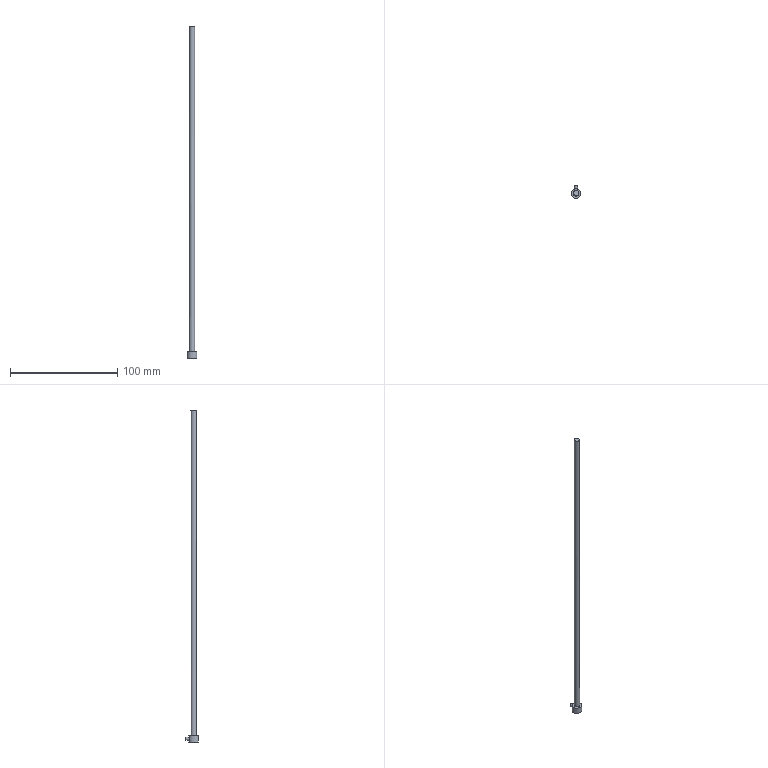Part | STEP file | E105-28-315 | 1 solid | 8 faces | box 9 x 12 x 309.813 mm | volume 6362 mm3 | cylinder 3 | plane 3 | spline 1 | cone 1 | commonest cylinder face diameters 3 x1 5 x1 9 x1
STEP:
#1=CARTESIAN_POINT('',(0.,0.,0.));
#2=DIRECTION('',(0.,0.,1.));
#3=DIRECTION('',(1.,0.,0.));
#4=AXIS2_PLACEMENT_3D('',#1,#2,#3);
#5=CARTESIAN_POINT('',(2.481,-0.3051,309.227));
#6=VERTEX_POINT('',#5);
#7=CARTESIAN_POINT('',(-2.5,0.,309.797));
#8=VERTEX_POINT('',#7);
#9=CARTESIAN_POINT('',(2.481,-0.3051,309.227));
#10=CARTESIAN_POINT('',(2.447,-0.5829,309.241));
#11=CARTESIAN_POINT('',(2.365,-0.8583,309.262));
#12=CARTESIAN_POINT('',(2.241,-1.109,309.287));
#13=CARTESIAN_POINT('',(2.117,-1.359,309.312));
#14=CARTESIAN_POINT('',(1.949,-1.591,309.342));
#15=CARTESIAN_POINT('',(1.75,-1.785,309.374));
#16=CARTESIAN_POINT('',(1.55,-1.982,309.406));
#17=CARTESIAN_POINT('',(1.313,-2.145,309.441));
#18=CARTESIAN_POINT('',(1.06,-2.264,309.476));
#19=CARTESIAN_POINT('',(0.8051,-2.383,309.511));
#20=CARTESIAN_POINT('',(0.526,-2.46,309.547));
#21=CARTESIAN_POINT('',(0.2457,-2.488,309.581));
#22=CARTESIAN_POINT('',(-0.03504,-2.516,309.615));
#23=CARTESIAN_POINT('',(-0.3247,-2.495,309.648));
#24=CARTESIAN_POINT('',(-0.5991,-2.427,309.677));
#25=CARTESIAN_POINT('',(-0.8724,-2.36,309.706));
#26=CARTESIAN_POINT('',(-1.138,-2.244,309.732));
#27=CARTESIAN_POINT('',(-1.374,-2.089,309.752));
#28=CARTESIAN_POINT('',(-1.608,-1.935,309.773));
#29=CARTESIAN_POINT('',(-1.819,-1.738,309.788));
#30=CARTESIAN_POINT('',(-1.989,-1.514,309.799));
#31=CARTESIAN_POINT('',(-2.158,-1.292,309.809));
#32=CARTESIAN_POINT('',(-2.291,-1.038,309.813));
#33=CARTESIAN_POINT('',(-2.378,-0.7725,309.813));
#34=CARTESIAN_POINT('',(-2.464,-0.508,309.812));
#35=CARTESIAN_POINT('',(-2.505,-0.2252,309.806));
#36=CARTESIAN_POINT('',(-2.499,0.05265,309.795));
#37=CARTESIAN_POINT('',(-2.494,0.3306,309.784));
#38=CARTESIAN_POINT('',(-2.44,0.6111,309.767));
#39=CARTESIAN_POINT('',(-2.343,0.8711,309.747));
#40=CARTESIAN_POINT('',(-2.246,1.132,309.727));
#41=CARTESIAN_POINT('',(-2.103,1.38,309.702));
#42=CARTESIAN_POINT('',(-1.926,1.594,309.674));
#43=CARTESIAN_POINT('',(-1.748,1.81,309.646));
#44=CARTESIAN_POINT('',(-1.53,1.997,309.615));
#45=CARTESIAN_POINT('',(-1.291,2.141,309.583));
#46=CARTESIAN_POINT('',(-1.05,2.286,309.551));
#47=CARTESIAN_POINT('',(-0.7814,2.391,309.516));
#48=CARTESIAN_POINT('',(-0.5065,2.448,309.482));
#49=CARTESIAN_POINT('',(-0.2307,2.505,309.449));
#50=CARTESIAN_POINT('',(0.05893,2.515,309.414));
#51=CARTESIAN_POINT('',(0.3383,2.477,309.383));
#52=CARTESIAN_POINT('',(0.6175,2.439,309.351));
#53=CARTESIAN_POINT('',(0.8943,2.352,309.322));
#54=CARTESIAN_POINT('',(1.145,2.222,309.296));
#55=CARTESIAN_POINT('',(1.395,2.093,309.271));
#56=CARTESIAN_POINT('',(1.627,1.919,309.249));
#57=CARTESIAN_POINT('',(1.82,1.714,309.233));
#58=CARTESIAN_POINT('',(2.011,1.511,309.217));
#59=CARTESIAN_POINT('',(2.171,1.271,309.206));
#60=CARTESIAN_POINT('',(2.285,1.015,309.201));
#61=CARTESIAN_POINT('',(2.398,0.7607,309.197));
#62=CARTESIAN_POINT('',(2.469,0.4835,309.198));
#63=CARTESIAN_POINT('',(2.491,0.2063,309.206));
#64=CARTESIAN_POINT('',(2.506,0.0363,309.211));
#65=CARTESIAN_POINT('',(2.502,-0.136,309.218));
#66=CARTESIAN_POINT('',(2.481,-0.3051,309.227));
#67=B_SPLINE_CURVE_WITH_KNOTS('',3,(#9,#10,#11,#12,#13,#14,#15,#16,#17,#18,#19,#20,#21,#22,#23,#24,#25,#26,#27,#28,#29,#30,#31,#32,#33,#34,#35,#36,#37,#38,#39,#40,#41,#42,#43,#44,#45,#46,#47,#48,#49,#50,#51,#52,#53,#54,#55,#56,#57,#58,#59,#60,#61,#62,#63,#64,#65,#66),.UNSPECIFIED.,.T.,.F.,(1,3,3,3,3,3,3,3,3,3,3,3,3,3,3,3,3,3,3,3,3,1),(-0.03233,0.,0.0536,0.1072,0.1611,0.2153,0.2697,0.3238,0.3775,0.4309,0.4841,0.5372,0.5907,0.6444,0.6984,0.7527,0.8069,0.8609,0.9145,0.9677,1.,1.054),.UNSPECIFIED.);
#68=CARTESIAN_POINT('',(0.,0.,106.));
#69=DIRECTION('',(0.,0.,-1.));
#70=DIRECTION('',(-1.,0.,0.));
#71=AXIS2_PLACEMENT_3D('',#68,#69,#70);
#72=CYLINDRICAL_SURFACE('',#71,2.5);
#73=CARTESIAN_POINT('',(3.264,-203.227));
#74=CARTESIAN_POINT('',(3.288,-203.23));
#75=CARTESIAN_POINT('',(3.335,-203.237));
#76=CARTESIAN_POINT('',(3.407,-203.248));
#77=CARTESIAN_POINT('',(3.479,-203.261));
#78=CARTESIAN_POINT('',(3.55,-203.276));
#79=CARTESIAN_POINT('',(3.621,-203.291));
#80=CARTESIAN_POINT('',(3.692,-203.308));
#81=CARTESIAN_POINT('',(3.764,-203.326));
#82=CARTESIAN_POINT('',(3.835,-203.345));
#83=CARTESIAN_POINT('',(3.907,-203.365));
#84=CARTESIAN_POINT('',(3.977,-203.385));
#85=CARTESIAN_POINT('',(4.049,-203.406));
#86=CARTESIAN_POINT('',(4.12,-203.428));
#87=CARTESIAN_POINT('',(4.191,-203.45));
#88=CARTESIAN_POINT('',(4.262,-203.472));
#89=CARTESIAN_POINT('',(4.333,-203.494));
#90=CARTESIAN_POINT('',(4.404,-203.516));
#91=CARTESIAN_POINT('',(4.475,-203.539));
#92=CARTESIAN_POINT('',(4.547,-203.561));
#93=CARTESIAN_POINT('',(4.618,-203.582));
#94=CARTESIAN_POINT('',(4.689,-203.604));
#95=CARTESIAN_POINT('',(4.76,-203.624));
#96=CARTESIAN_POINT('',(4.831,-203.645));
#97=CARTESIAN_POINT('',(4.903,-203.664));
#98=CARTESIAN_POINT('',(4.973,-203.682));
#99=CARTESIAN_POINT('',(5.045,-203.7));
#100=CARTESIAN_POINT('',(5.116,-203.716));
#101=CARTESIAN_POINT('',(5.188,-203.732));
#102=CARTESIAN_POINT('',(5.259,-203.746));
#103=CARTESIAN_POINT('',(5.33,-203.759));
#104=CARTESIAN_POINT('',(5.402,-203.77));
#105=CARTESIAN_POINT('',(5.474,-203.781));
#106=CARTESIAN_POINT('',(5.545,-203.79));
#107=CARTESIAN_POINT('',(5.617,-203.797));
#108=CARTESIAN_POINT('',(5.688,-203.803));
#109=CARTESIAN_POINT('',(5.76,-203.808));
#110=CARTESIAN_POINT('',(5.832,-203.811));
#111=CARTESIAN_POINT('',(5.903,-203.813));
#112=CARTESIAN_POINT('',(5.975,-203.813));
#113=CARTESIAN_POINT('',(6.046,-203.812));
#114=CARTESIAN_POINT('',(6.118,-203.809));
#115=CARTESIAN_POINT('',(6.19,-203.805));
#116=CARTESIAN_POINT('',(6.262,-203.799));
#117=CARTESIAN_POINT('',(6.333,-203.792));
#118=CARTESIAN_POINT('',(6.404,-203.784));
#119=CARTESIAN_POINT('',(6.476,-203.774));
#120=CARTESIAN_POINT('',(6.548,-203.763));
#121=CARTESIAN_POINT('',(6.619,-203.751));
#122=CARTESIAN_POINT('',(6.69,-203.737));
#123=CARTESIAN_POINT('',(6.762,-203.723));
#124=CARTESIAN_POINT('',(6.834,-203.708));
#125=CARTESIAN_POINT('',(6.905,-203.691));
#126=CARTESIAN_POINT('',(6.976,-203.674));
#127=CARTESIAN_POINT('',(7.047,-203.656));
#128=CARTESIAN_POINT('',(7.119,-203.637));
#129=CARTESIAN_POINT('',(7.19,-203.617));
#130=CARTESIAN_POINT('',(7.261,-203.597));
#131=CARTESIAN_POINT('',(7.332,-203.577));
#132=CARTESIAN_POINT('',(7.403,-203.556));
#133=CARTESIAN_POINT('',(7.475,-203.535));
#134=CARTESIAN_POINT('',(7.546,-203.514));
#135=CARTESIAN_POINT('',(7.617,-203.492));
#136=CARTESIAN_POINT('',(7.688,-203.471));
#137=CARTESIAN_POINT('',(7.759,-203.45));
#138=CARTESIAN_POINT('',(7.83,-203.429));
#139=CARTESIAN_POINT('',(7.902,-203.408));
#140=CARTESIAN_POINT('',(7.973,-203.387));
#141=CARTESIAN_POINT('',(8.044,-203.368));
#142=CARTESIAN_POINT('',(8.115,-203.349));
#143=CARTESIAN_POINT('',(8.187,-203.33));
#144=CARTESIAN_POINT('',(8.258,-203.313));
#145=CARTESIAN_POINT('',(8.329,-203.296));
#146=CARTESIAN_POINT('',(8.4,-203.28));
#147=CARTESIAN_POINT('',(8.472,-203.266));
#148=CARTESIAN_POINT('',(8.544,-203.253));
#149=CARTESIAN_POINT('',(8.615,-203.241));
#150=CARTESIAN_POINT('',(8.686,-203.23));
#151=CARTESIAN_POINT('',(8.758,-203.221));
#152=CARTESIAN_POINT('',(8.83,-203.213));
#153=CARTESIAN_POINT('',(8.901,-203.207));
#154=CARTESIAN_POINT('',(8.973,-203.203));
#155=CARTESIAN_POINT('',(9.044,-203.2));
#156=CARTESIAN_POINT('',(9.116,-203.199));
#157=CARTESIAN_POINT('',(9.188,-203.199));
#158=CARTESIAN_POINT('',(9.26,-203.201));
#159=CARTESIAN_POINT('',(9.331,-203.205));
#160=CARTESIAN_POINT('',(9.403,-203.21));
#161=CARTESIAN_POINT('',(9.475,-203.218));
#162=CARTESIAN_POINT('',(9.523,-203.223));
#163=CARTESIAN_POINT('',(9.547,-203.227));
#164=B_SPLINE_CURVE_WITH_KNOTS('',3,(#73,#74,#75,#76,#77,#78,#79,#80,#81,#82,#83,#84,#85,#86,#87,#88,#89,#90,#91,#92,#93,#94,#95,#96,#97,#98,#99,#100,#101,#102,#103,#104,#105,#106,#107,#108,#109,#110,#111,#112,#113,#114,#115,#116,#117,#118,#119,#120,#121,#122,#123,#124,#125,#126,#127,#128,#129,#130,#131,#132,#133,#134,#135,#136,#137,#138,#139,#140,#141,#142,#143,#144,#145,#146,#147,#148,#149,#150,#151,#152,#153,#154,#155,#156,#157,#158,#159,#160,#161,#162,#163),.UNSPECIFIED.,.F.,.F.,(4,1,1,1,1,1,1,1,1,1,1,1,1,1,1,1,1,1,1,1,1,1,1,1,1,1,1,1,1,1,1,1,1,1,1,1,1,1,1,1,1,1,1,1,1,1,1,1,1,1,1,1,1,1,1,1,1,1,1,1,1,1,1,1,1,1,1,1,1,1,1,1,1,1,1,1,1,1,1,1,1,1,1,1,1,1,1,1,4),(0.,0.01136,0.02273,0.03409,0.04545,0.05682,0.06818,0.07955,0.09091,0.1023,0.1136,0.125,0.1364,0.1477,0.1591,0.1705,0.1818,0.1932,0.2045,0.2159,0.2273,0.2386,0.25,0.2614,0.2727,0.2841,0.2955,0.3068,0.3182,0.3295,0.3409,0.3523,0.3636,0.375,0.3864,0.3977,0.4091,0.4205,0.4318,0.4432,0.4545,0.4659,0.4773,0.4886,0.5,0.5114,0.5227,0.5341,0.5455,0.5568,0.5682,0.5795,0.5909,0.6023,0.6136,0.625,0.6364,0.6477,0.6591,0.6705,0.6818,0.6932,0.7045,0.7159,0.7273,0.7386,0.75,0.7614,0.7727,0.7841,0.7955,0.8068,0.8182,0.8295,0.8409,0.8523,0.8636,0.875,0.8864,0.8977,0.9091,0.9205,0.9318,0.9432,0.9545,0.9659,0.9773,0.9886,1.),.QUASI_UNIFORM_KNOTS.);
#165=(GEOMETRIC_REPRESENTATION_CONTEXT(2)PARAMETRIC_REPRESENTATION_CONTEXT()REPRESENTATION_CONTEXT('',''));
#166=DEFINITIONAL_REPRESENTATION('',(#164),#165);
#167=PCURVE('',#72,#166);
#168=CARTESIAN_POINT('',(-12.541,-3.319,310.811));
#169=CARTESIAN_POINT('',(-7.15,-3.317,310.438));
#170=CARTESIAN_POINT('',(-1.699,-3.315,309.89));
#171=CARTESIAN_POINT('',(3.819,-3.313,309.168));
#172=CARTESIAN_POINT('',(-12.563,-0.6316,310.712));
#173=CARTESIAN_POINT('',(-7.174,-0.6296,310.339));
#174=CARTESIAN_POINT('',(-1.725,-0.6278,309.792));
#175=CARTESIAN_POINT('',(3.791,-0.6259,309.071));
#176=CARTESIAN_POINT('',(-12.586,2.055,310.611));
#177=CARTESIAN_POINT('',(-7.199,2.057,310.239));
#178=CARTESIAN_POINT('',(-1.752,2.059,309.693));
#179=CARTESIAN_POINT('',(3.762,2.061,308.973));
#180=CARTESIAN_POINT('',(-12.61,4.742,310.511));
#181=CARTESIAN_POINT('',(-7.225,4.744,310.139));
#182=CARTESIAN_POINT('',(-1.78,4.746,309.594));
#183=CARTESIAN_POINT('',(3.733,4.748,308.875));
#184=B_SPLINE_SURFACE_WITH_KNOTS('',3,3,((#168,#169,#170,#171),(#172,#173,#174,#175),(#176,#177,#178,#179),(#180,#181,#182,#183)),.UNSPECIFIED.,.F.,.F.,.F.,(4,4),(4,4),(0.,1.),(0.,1.),.PIECEWISE_BEZIER_KNOTS.);
#185=CARTESIAN_POINT('',(0.3732,0.921));
#186=CARTESIAN_POINT('',(0.3662,0.9205));
#187=CARTESIAN_POINT('',(0.3521,0.9194));
#188=CARTESIAN_POINT('',(0.3313,0.9169));
#189=CARTESIAN_POINT('',(0.3109,0.9138));
#190=CARTESIAN_POINT('',(0.2909,0.91));
#191=CARTESIAN_POINT('',(0.2716,0.9056));
#192=CARTESIAN_POINT('',(0.253,0.9005));
#193=CARTESIAN_POINT('',(0.2351,0.8948));
#194=CARTESIAN_POINT('',(0.2179,0.8885));
#195=CARTESIAN_POINT('',(0.2017,0.8817));
#196=CARTESIAN_POINT('',(0.1866,0.8744));
#197=CARTESIAN_POINT('',(0.1725,0.8666));
#198=CARTESIAN_POINT('',(0.1595,0.8583));
#199=CARTESIAN_POINT('',(0.1476,0.8496));
#200=CARTESIAN_POINT('',(0.137,0.8406));
#201=CARTESIAN_POINT('',(0.1277,0.8313));
#202=CARTESIAN_POINT('',(0.1198,0.8216));
#203=CARTESIAN_POINT('',(0.1132,0.8117));
#204=CARTESIAN_POINT('',(0.1079,0.8016));
#205=CARTESIAN_POINT('',(0.1041,0.7914));
#206=CARTESIAN_POINT('',(0.1017,0.7811));
#207=CARTESIAN_POINT('',(0.1008,0.7707));
#208=CARTESIAN_POINT('',(0.1013,0.7603));
#209=CARTESIAN_POINT('',(0.1033,0.7499));
#210=CARTESIAN_POINT('',(0.1067,0.7397));
#211=CARTESIAN_POINT('',(0.1115,0.7296));
#212=CARTESIAN_POINT('',(0.1178,0.7197));
#213=CARTESIAN_POINT('',(0.1254,0.7099));
#214=CARTESIAN_POINT('',(0.1344,0.7005));
#215=CARTESIAN_POINT('',(0.1447,0.6914));
#216=CARTESIAN_POINT('',(0.1562,0.6827));
#217=CARTESIAN_POINT('',(0.169,0.6743));
#218=CARTESIAN_POINT('',(0.1829,0.6665));
#219=CARTESIAN_POINT('',(0.198,0.659));
#220=CARTESIAN_POINT('',(0.214,0.6522));
#221=CARTESIAN_POINT('',(0.2308,0.6459));
#222=CARTESIAN_POINT('',(0.2487,0.6402));
#223=CARTESIAN_POINT('',(0.2673,0.6351));
#224=CARTESIAN_POINT('',(0.2866,0.6306));
#225=CARTESIAN_POINT('',(0.3065,0.6268));
#226=CARTESIAN_POINT('',(0.3267,0.6237));
#227=CARTESIAN_POINT('',(0.3475,0.6213));
#228=CARTESIAN_POINT('',(0.3686,0.6196));
#229=CARTESIAN_POINT('',(0.3899,0.6186));
#230=CARTESIAN_POINT('',(0.4042,0.6185));
#231=CARTESIAN_POINT('',(0.4113,0.6185));
#232=B_SPLINE_CURVE_WITH_KNOTS('',3,(#185,#186,#187,#188,#189,#190,#191,#192,#193,#194,#195,#196,#197,#198,#199,#200,#201,#202,#203,#204,#205,#206,#207,#208,#209,#210,#211,#212,#213,#214,#215,#216,#217,#218,#219,#220,#221,#222,#223,#224,#225,#226,#227,#228,#229,#230,#231),.UNSPECIFIED.,.F.,.F.,(4,1,1,1,1,1,1,1,1,1,1,1,1,1,1,1,1,1,1,1,1,1,1,1,1,1,1,1,1,1,1,1,1,1,1,1,1,1,1,1,1,1,1,1,4),(0.,0.01093,0.02185,0.03278,0.0437,0.05463,0.06555,0.07648,0.0874,0.09833,0.1093,0.1202,0.1311,0.142,0.153,0.1639,0.1748,0.1857,0.1967,0.2076,0.2185,0.2294,0.2404,0.2513,0.2622,0.2731,0.2841,0.295,0.3059,0.3168,0.3278,0.3387,0.3496,0.3605,0.3715,0.3824,0.3933,0.4042,0.4152,0.4261,0.437,0.4479,0.4589,0.4698,0.4807),.QUASI_UNIFORM_KNOTS.);
#233=(GEOMETRIC_REPRESENTATION_CONTEXT(2)PARAMETRIC_REPRESENTATION_CONTEXT()REPRESENTATION_CONTEXT('',''));
#234=DEFINITIONAL_REPRESENTATION('',(#232),#233);
#235=PCURVE('',#184,#234);
#236=SURFACE_CURVE('',#67,(#167,#235),.PCURVE_S1.);
#237=EDGE_CURVE('',#6,#8,#236,.T.);
#238=ORIENTED_EDGE('',*,*,#237,.T.);
#239=CARTESIAN_POINT('',(-2.5,0.,6.));
#240=VERTEX_POINT('',#239);
#241=CARTESIAN_POINT('',(-2.5,0.,309.797));
#242=CARTESIAN_POINT('',(-2.5,0.,6.));
#243=B_SPLINE_CURVE_WITH_KNOTS('',1,(#241,#242),.UNSPECIFIED.,.F.,.F.,(2,2),(-203.797,100.),.PIECEWISE_BEZIER_KNOTS.);
#244=CARTESIAN_POINT('',(6.283,0.));
#245=DIRECTION('',(0.,1.));
#246=VECTOR('',#245,1.);
#247=LINE('',#244,#246);
#248=(GEOMETRIC_REPRESENTATION_CONTEXT(2)PARAMETRIC_REPRESENTATION_CONTEXT()REPRESENTATION_CONTEXT('',''));
#249=DEFINITIONAL_REPRESENTATION('',(#247),#248);
#250=PCURVE('',#72,#249);
#251=CARTESIAN_POINT('',(0.,0.));
#252=DIRECTION('',(0.,1.));
#253=VECTOR('',#252,1.);
#254=LINE('',#251,#253);
#255=(GEOMETRIC_REPRESENTATION_CONTEXT(2)PARAMETRIC_REPRESENTATION_CONTEXT()REPRESENTATION_CONTEXT('',''));
#256=DEFINITIONAL_REPRESENTATION('',(#254),#255);
#257=PCURVE('',#72,#256);
#258=SEAM_CURVE('',#243,(#250,#257),.PCURVE_S1.);
#259=EDGE_CURVE('',#8,#240,#258,.T.);
#260=ORIENTED_EDGE('',*,*,#259,.T.);
#261=CARTESIAN_POINT('',(0.,0.,6.));
#262=DIRECTION('',(0.,0.,-1.));
#263=DIRECTION('',(-1.,0.,0.));
#264=AXIS2_PLACEMENT_3D('',#261,#262,#263);
#265=CIRCLE('',#264,2.5);
#266=CARTESIAN_POINT('',(0.,100.));
#267=DIRECTION('',(1.,0.));
#268=VECTOR('',#267,1.);
#269=LINE('',#266,#268);
#270=(GEOMETRIC_REPRESENTATION_CONTEXT(2)PARAMETRIC_REPRESENTATION_CONTEXT()REPRESENTATION_CONTEXT('',''));
#271=DEFINITIONAL_REPRESENTATION('',(#269),#270);
#272=PCURVE('',#72,#271);
#273=CARTESIAN_POINT('',(0.,0.,6.));
#274=DIRECTION('',(0.,0.,-1.));
#275=DIRECTION('',(1.,0.,0.));
#276=AXIS2_PLACEMENT_3D('',#273,#274,#275);
#277=PLANE('',#276);
#278=CARTESIAN_POINT('',(0.,0.));
#279=DIRECTION('',(-1.,0.));
#280=AXIS2_PLACEMENT_2D('',#278,#279);
#281=CIRCLE('',#280,2.5);
#282=(GEOMETRIC_REPRESENTATION_CONTEXT(2)PARAMETRIC_REPRESENTATION_CONTEXT()REPRESENTATION_CONTEXT('',''));
#283=DEFINITIONAL_REPRESENTATION('',(#281),#282);
#284=PCURVE('',#277,#283);
#285=SURFACE_CURVE('',#265,(#272,#284),.PCURVE_S1.);
#286=EDGE_CURVE('',#240,#240,#285,.T.);
#287=ORIENTED_EDGE('',*,*,#286,.F.);
#288=ORIENTED_EDGE('',*,*,#259,.F.);
#289=CARTESIAN_POINT('',(2.481,-0.3051,309.227));
#290=CARTESIAN_POINT('',(2.447,-0.5829,309.241));
#291=CARTESIAN_POINT('',(2.365,-0.8583,309.262));
#292=CARTESIAN_POINT('',(2.241,-1.109,309.287));
#293=CARTESIAN_POINT('',(2.117,-1.359,309.312));
#294=CARTESIAN_POINT('',(1.949,-1.591,309.342));
#295=CARTESIAN_POINT('',(1.75,-1.785,309.374));
#296=CARTESIAN_POINT('',(1.55,-1.982,309.406));
#297=CARTESIAN_POINT('',(1.313,-2.145,309.441));
#298=CARTESIAN_POINT('',(1.06,-2.264,309.476));
#299=CARTESIAN_POINT('',(0.8051,-2.383,309.511));
#300=CARTESIAN_POINT('',(0.526,-2.46,309.547));
#301=CARTESIAN_POINT('',(0.2457,-2.488,309.581));
#302=CARTESIAN_POINT('',(-0.03504,-2.516,309.615));
#303=CARTESIAN_POINT('',(-0.3247,-2.495,309.648));
#304=CARTESIAN_POINT('',(-0.5991,-2.427,309.677));
#305=CARTESIAN_POINT('',(-0.8724,-2.36,309.706));
#306=CARTESIAN_POINT('',(-1.138,-2.244,309.732));
#307=CARTESIAN_POINT('',(-1.374,-2.089,309.752));
#308=CARTESIAN_POINT('',(-1.608,-1.935,309.773));
#309=CARTESIAN_POINT('',(-1.819,-1.738,309.788));
#310=CARTESIAN_POINT('',(-1.989,-1.514,309.799));
#311=CARTESIAN_POINT('',(-2.158,-1.292,309.809));
#312=CARTESIAN_POINT('',(-2.291,-1.038,309.813));
#313=CARTESIAN_POINT('',(-2.378,-0.7725,309.813));
#314=CARTESIAN_POINT('',(-2.464,-0.508,309.812));
#315=CARTESIAN_POINT('',(-2.505,-0.2252,309.806));
#316=CARTESIAN_POINT('',(-2.499,0.05265,309.795));
#317=CARTESIAN_POINT('',(-2.494,0.3306,309.784));
#318=CARTESIAN_POINT('',(-2.44,0.6111,309.767));
#319=CARTESIAN_POINT('',(-2.343,0.8711,309.747));
#320=CARTESIAN_POINT('',(-2.246,1.132,309.727));
#321=CARTESIAN_POINT('',(-2.103,1.38,309.702));
#322=CARTESIAN_POINT('',(-1.926,1.594,309.674));
#323=CARTESIAN_POINT('',(-1.748,1.81,309.646));
#324=CARTESIAN_POINT('',(-1.53,1.997,309.615));
#325=CARTESIAN_POINT('',(-1.291,2.141,309.583));
#326=CARTESIAN_POINT('',(-1.05,2.286,309.551));
#327=CARTESIAN_POINT('',(-0.7814,2.391,309.516));
#328=CARTESIAN_POINT('',(-0.5065,2.448,309.482));
#329=CARTESIAN_POINT('',(-0.2307,2.505,309.449));
#330=CARTESIAN_POINT('',(0.05893,2.515,309.414));
#331=CARTESIAN_POINT('',(0.3383,2.477,309.383));
#332=CARTESIAN_POINT('',(0.6175,2.439,309.351));
#333=CARTESIAN_POINT('',(0.8943,2.352,309.322));
#334=CARTESIAN_POINT('',(1.145,2.222,309.296));
#335=CARTESIAN_POINT('',(1.395,2.093,309.271));
#336=CARTESIAN_POINT('',(1.627,1.919,309.249));
#337=CARTESIAN_POINT('',(1.82,1.714,309.233));
#338=CARTESIAN_POINT('',(2.011,1.511,309.217));
#339=CARTESIAN_POINT('',(2.171,1.271,309.206));
#340=CARTESIAN_POINT('',(2.285,1.015,309.201));
#341=CARTESIAN_POINT('',(2.398,0.7607,309.197));
#342=CARTESIAN_POINT('',(2.469,0.4835,309.198));
#343=CARTESIAN_POINT('',(2.491,0.2063,309.206));
#344=CARTESIAN_POINT('',(2.506,0.0363,309.211));
#345=CARTESIAN_POINT('',(2.502,-0.136,309.218));
#346=CARTESIAN_POINT('',(2.481,-0.3051,309.227));
#347=B_SPLINE_CURVE_WITH_KNOTS('',3,(#289,#290,#291,#292,#293,#294,#295,#296,#297,#298,#299,#300,#301,#302,#303,#304,#305,#306,#307,#308,#309,#310,#311,#312,#313,#314,#315,#316,#317,#318,#319,#320,#321,#322,#323,#324,#325,#326,#327,#328,#329,#330,#331,#332,#333,#334,#335,#336,#337,#338,#339,#340,#341,#342,#343,#344,#345,#346),.UNSPECIFIED.,.T.,.F.,(1,3,3,3,3,3,3,3,3,3,3,3,3,3,3,3,3,3,3,3,3,1),(-0.03233,0.,0.0536,0.1072,0.1611,0.2153,0.2697,0.3238,0.3775,0.4309,0.4841,0.5372,0.5907,0.6444,0.6984,0.7527,0.8069,0.8609,0.9145,0.9677,1.,1.054),.UNSPECIFIED.);
#348=CARTESIAN_POINT('',(-3.019,-203.227));
#349=CARTESIAN_POINT('',(-2.996,-203.23));
#350=CARTESIAN_POINT('',(-2.948,-203.237));
#351=CARTESIAN_POINT('',(-2.876,-203.248));
#352=CARTESIAN_POINT('',(-2.805,-203.261));
#353=CARTESIAN_POINT('',(-2.733,-203.276));
#354=CARTESIAN_POINT('',(-2.662,-203.291));
#355=CARTESIAN_POINT('',(-2.591,-203.308));
#356=CARTESIAN_POINT('',(-2.519,-203.326));
#357=CARTESIAN_POINT('',(-2.448,-203.345));
#358=CARTESIAN_POINT('',(-2.377,-203.365));
#359=CARTESIAN_POINT('',(-2.306,-203.385));
#360=CARTESIAN_POINT('',(-2.235,-203.406));
#361=CARTESIAN_POINT('',(-2.163,-203.428));
#362=CARTESIAN_POINT('',(-2.092,-203.45));
#363=CARTESIAN_POINT('',(-2.021,-203.472));
#364=CARTESIAN_POINT('',(-1.95,-203.494));
#365=CARTESIAN_POINT('',(-1.879,-203.516));
#366=CARTESIAN_POINT('',(-1.808,-203.539));
#367=CARTESIAN_POINT('',(-1.736,-203.561));
#368=CARTESIAN_POINT('',(-1.666,-203.582));
#369=CARTESIAN_POINT('',(-1.595,-203.604));
#370=CARTESIAN_POINT('',(-1.523,-203.624));
#371=CARTESIAN_POINT('',(-1.452,-203.645));
#372=CARTESIAN_POINT('',(-1.381,-203.664));
#373=CARTESIAN_POINT('',(-1.31,-203.682));
#374=CARTESIAN_POINT('',(-1.238,-203.7));
#375=CARTESIAN_POINT('',(-1.167,-203.716));
#376=CARTESIAN_POINT('',(-1.095,-203.732));
#377=CARTESIAN_POINT('',(-1.024,-203.746));
#378=CARTESIAN_POINT('',(-0.9529,-203.759));
#379=CARTESIAN_POINT('',(-0.8813,-203.77));
#380=CARTESIAN_POINT('',(-0.8096,-203.781));
#381=CARTESIAN_POINT('',(-0.7379,-203.79));
#382=CARTESIAN_POINT('',(-0.6664,-203.797));
#383=CARTESIAN_POINT('',(-0.5951,-203.803));
#384=CARTESIAN_POINT('',(-0.5234,-203.808));
#385=CARTESIAN_POINT('',(-0.4515,-203.811));
#386=CARTESIAN_POINT('',(-0.3797,-203.813));
#387=CARTESIAN_POINT('',(-0.3084,-203.813));
#388=CARTESIAN_POINT('',(-0.2369,-203.812));
#389=CARTESIAN_POINT('',(-0.165,-203.809));
#390=CARTESIAN_POINT('',(-0.09322,-203.805));
#391=CARTESIAN_POINT('',(-0.02151,-203.799));
#392=CARTESIAN_POINT('',(0.04972,-203.792));
#393=CARTESIAN_POINT('',(0.1213,-203.784));
#394=CARTESIAN_POINT('',(0.193,-203.774));
#395=CARTESIAN_POINT('',(0.2647,-203.763));
#396=CARTESIAN_POINT('',(0.3362,-203.751));
#397=CARTESIAN_POINT('',(0.4073,-203.737));
#398=CARTESIAN_POINT('',(0.4788,-203.723));
#399=CARTESIAN_POINT('',(0.5504,-203.708));
#400=CARTESIAN_POINT('',(0.6219,-203.691));
#401=CARTESIAN_POINT('',(0.693,-203.674));
#402=CARTESIAN_POINT('',(0.7641,-203.656));
#403=CARTESIAN_POINT('',(0.8355,-203.637));
#404=CARTESIAN_POINT('',(0.907,-203.617));
#405=CARTESIAN_POINT('',(0.9783,-203.597));
#406=CARTESIAN_POINT('',(1.049,-203.577));
#407=CARTESIAN_POINT('',(1.12,-203.556));
#408=CARTESIAN_POINT('',(1.192,-203.535));
#409=CARTESIAN_POINT('',(1.263,-203.514));
#410=CARTESIAN_POINT('',(1.334,-203.492));
#411=CARTESIAN_POINT('',(1.405,-203.471));
#412=CARTESIAN_POINT('',(1.476,-203.45));
#413=CARTESIAN_POINT('',(1.547,-203.429));
#414=CARTESIAN_POINT('',(1.619,-203.408));
#415=CARTESIAN_POINT('',(1.69,-203.387));
#416=CARTESIAN_POINT('',(1.761,-203.368));
#417=CARTESIAN_POINT('',(1.832,-203.349));
#418=CARTESIAN_POINT('',(1.903,-203.33));
#419=CARTESIAN_POINT('',(1.975,-203.313));
#420=CARTESIAN_POINT('',(2.046,-203.296));
#421=CARTESIAN_POINT('',(2.117,-203.28));
#422=CARTESIAN_POINT('',(2.189,-203.266));
#423=CARTESIAN_POINT('',(2.26,-203.253));
#424=CARTESIAN_POINT('',(2.332,-203.241));
#425=CARTESIAN_POINT('',(2.403,-203.23));
#426=CARTESIAN_POINT('',(2.475,-203.221));
#427=CARTESIAN_POINT('',(2.546,-203.213));
#428=CARTESIAN_POINT('',(2.618,-203.207));
#429=CARTESIAN_POINT('',(2.69,-203.203));
#430=CARTESIAN_POINT('',(2.761,-203.2));
#431=CARTESIAN_POINT('',(2.833,-203.199));
#432=CARTESIAN_POINT('',(2.905,-203.199));
#433=CARTESIAN_POINT('',(2.976,-203.201));
#434=CARTESIAN_POINT('',(3.048,-203.205));
#435=CARTESIAN_POINT('',(3.12,-203.21));
#436=CARTESIAN_POINT('',(3.192,-203.218));
#437=CARTESIAN_POINT('',(3.24,-203.223));
#438=CARTESIAN_POINT('',(3.264,-203.227));
#439=B_SPLINE_CURVE_WITH_KNOTS('',3,(#348,#349,#350,#351,#352,#353,#354,#355,#356,#357,#358,#359,#360,#361,#362,#363,#364,#365,#366,#367,#368,#369,#370,#371,#372,#373,#374,#375,#376,#377,#378,#379,#380,#381,#382,#383,#384,#385,#386,#387,#388,#389,#390,#391,#392,#393,#394,#395,#396,#397,#398,#399,#400,#401,#402,#403,#404,#405,#406,#407,#408,#409,#410,#411,#412,#413,#414,#415,#416,#417,#418,#419,#420,#421,#422,#423,#424,#425,#426,#427,#428,#429,#430,#431,#432,#433,#434,#435,#436,#437,#438),.UNSPECIFIED.,.F.,.F.,(4,1,1,1,1,1,1,1,1,1,1,1,1,1,1,1,1,1,1,1,1,1,1,1,1,1,1,1,1,1,1,1,1,1,1,1,1,1,1,1,1,1,1,1,1,1,1,1,1,1,1,1,1,1,1,1,1,1,1,1,1,1,1,1,1,1,1,1,1,1,1,1,1,1,1,1,1,1,1,1,1,1,1,1,1,1,1,1,4),(0.,0.01136,0.02273,0.03409,0.04545,0.05682,0.06818,0.07955,0.09091,0.1023,0.1136,0.125,0.1364,0.1477,0.1591,0.1705,0.1818,0.1932,0.2045,0.2159,0.2273,0.2386,0.25,0.2614,0.2727,0.2841,0.2955,0.3068,0.3182,0.3295,0.3409,0.3523,0.3636,0.375,0.3864,0.3977,0.4091,0.4205,0.4318,0.4432,0.4545,0.4659,0.4773,0.4886,0.5,0.5114,0.5227,0.5341,0.5455,0.5568,0.5682,0.5795,0.5909,0.6023,0.6136,0.625,0.6364,0.6477,0.6591,0.6705,0.6818,0.6932,0.7045,0.7159,0.7273,0.7386,0.75,0.7614,0.7727,0.7841,0.7955,0.8068,0.8182,0.8295,0.8409,0.8523,0.8636,0.875,0.8864,0.8977,0.9091,0.9205,0.9318,0.9432,0.9545,0.9659,0.9773,0.9886,1.),.QUASI_UNIFORM_KNOTS.);
#440=(GEOMETRIC_REPRESENTATION_CONTEXT(2)PARAMETRIC_REPRESENTATION_CONTEXT()REPRESENTATION_CONTEXT('',''));
#441=DEFINITIONAL_REPRESENTATION('',(#439),#440);
#442=PCURVE('',#72,#441);
#443=CARTESIAN_POINT('',(0.4113,0.6185));
#444=CARTESIAN_POINT('',(0.4189,0.6185));
#445=CARTESIAN_POINT('',(0.4342,0.6189));
#446=CARTESIAN_POINT('',(0.4572,0.6203));
#447=CARTESIAN_POINT('',(0.4799,0.6225));
#448=CARTESIAN_POINT('',(0.5022,0.6255));
#449=CARTESIAN_POINT('',(0.5239,0.6293));
#450=CARTESIAN_POINT('',(0.545,0.6339));
#451=CARTESIAN_POINT('',(0.5654,0.6393));
#452=CARTESIAN_POINT('',(0.585,0.6453));
#453=CARTESIAN_POINT('',(0.6036,0.6521));
#454=CARTESIAN_POINT('',(0.621,0.6595));
#455=CARTESIAN_POINT('',(0.6373,0.6675));
#456=CARTESIAN_POINT('',(0.6525,0.6761));
#457=CARTESIAN_POINT('',(0.6663,0.6852));
#458=CARTESIAN_POINT('',(0.6786,0.6947));
#459=CARTESIAN_POINT('',(0.6895,0.7046));
#460=CARTESIAN_POINT('',(0.6989,0.715));
#461=CARTESIAN_POINT('',(0.7067,0.7256));
#462=CARTESIAN_POINT('',(0.7129,0.7365));
#463=CARTESIAN_POINT('',(0.7174,0.7475));
#464=CARTESIAN_POINT('',(0.7203,0.7586));
#465=CARTESIAN_POINT('',(0.7215,0.7699));
#466=CARTESIAN_POINT('',(0.721,0.7811));
#467=CARTESIAN_POINT('',(0.7188,0.7923));
#468=CARTESIAN_POINT('',(0.715,0.8033));
#469=CARTESIAN_POINT('',(0.7094,0.8142));
#470=CARTESIAN_POINT('',(0.7022,0.8249));
#471=CARTESIAN_POINT('',(0.6934,0.8353));
#472=CARTESIAN_POINT('',(0.6832,0.8452));
#473=CARTESIAN_POINT('',(0.6713,0.8548));
#474=CARTESIAN_POINT('',(0.658,0.864));
#475=CARTESIAN_POINT('',(0.6434,0.8726));
#476=CARTESIAN_POINT('',(0.6275,0.8807));
#477=CARTESIAN_POINT('',(0.6104,0.8881));
#478=CARTESIAN_POINT('',(0.5922,0.8949));
#479=CARTESIAN_POINT('',(0.5729,0.9011));
#480=CARTESIAN_POINT('',(0.5527,0.9065));
#481=CARTESIAN_POINT('',(0.5319,0.9111));
#482=CARTESIAN_POINT('',(0.5103,0.915));
#483=CARTESIAN_POINT('',(0.4881,0.9181));
#484=CARTESIAN_POINT('',(0.4655,0.9204));
#485=CARTESIAN_POINT('',(0.4427,0.9218));
#486=CARTESIAN_POINT('',(0.4195,0.9224));
#487=CARTESIAN_POINT('',(0.3963,0.9222));
#488=CARTESIAN_POINT('',(0.3808,0.9215));
#489=CARTESIAN_POINT('',(0.3732,0.921));
#490=B_SPLINE_CURVE_WITH_KNOTS('',3,(#443,#444,#445,#446,#447,#448,#449,#450,#451,#452,#453,#454,#455,#456,#457,#458,#459,#460,#461,#462,#463,#464,#465,#466,#467,#468,#469,#470,#471,#472,#473,#474,#475,#476,#477,#478,#479,#480,#481,#482,#483,#484,#485,#486,#487,#488,#489),.UNSPECIFIED.,.F.,.F.,(4,1,1,1,1,1,1,1,1,1,1,1,1,1,1,1,1,1,1,1,1,1,1,1,1,1,1,1,1,1,1,1,1,1,1,1,1,1,1,1,1,1,1,1,4),(0.4807,0.4925,0.5043,0.5161,0.5279,0.5397,0.5515,0.5633,0.5751,0.5869,0.5987,0.6105,0.6223,0.6341,0.6459,0.6577,0.6695,0.6813,0.6931,0.7049,0.7168,0.7286,0.7404,0.7522,0.764,0.7758,0.7876,0.7994,0.8112,0.823,0.8348,0.8466,0.8584,0.8702,0.882,0.8938,0.9056,0.9174,0.9292,0.941,0.9528,0.9646,0.9764,0.9882,1.),.QUASI_UNIFORM_KNOTS.);
#491=(GEOMETRIC_REPRESENTATION_CONTEXT(2)PARAMETRIC_REPRESENTATION_CONTEXT()REPRESENTATION_CONTEXT('',''));
#492=DEFINITIONAL_REPRESENTATION('',(#490),#491);
#493=PCURVE('',#184,#492);
#494=SURFACE_CURVE('',#347,(#442,#493),.PCURVE_S1.);
#495=EDGE_CURVE('',#8,#6,#494,.T.);
#496=ORIENTED_EDGE('',*,*,#495,.T.);
#497=EDGE_LOOP('',(#238,#260,#287,#288,#496));
#498=FACE_BOUND('',#497,.T.);
#499=ADVANCED_FACE('',(#498),#72,.T.);
#500=ORIENTED_EDGE('',*,*,#495,.T.);
#501=ORIENTED_EDGE('',*,*,#237,.T.);
#502=EDGE_LOOP('',(#500,#501));
#503=FACE_BOUND('',#502,.F.);
#504=ADVANCED_FACE('',(#503),#184,.F.);
#505=CARTESIAN_POINT('',(-4.5,0.,6.));
#506=VERTEX_POINT('',#505);
#507=CARTESIAN_POINT('',(0.,0.,6.));
#508=DIRECTION('',(0.,0.,-1.));
#509=DIRECTION('',(-1.,0.,0.));
#510=AXIS2_PLACEMENT_3D('',#507,#508,#509);
#511=CIRCLE('',#510,4.5);
#512=CARTESIAN_POINT('',(0.,0.));
#513=DIRECTION('',(-1.,0.));
#514=AXIS2_PLACEMENT_2D('',#512,#513);
#515=CIRCLE('',#514,4.5);
#516=(GEOMETRIC_REPRESENTATION_CONTEXT(2)PARAMETRIC_REPRESENTATION_CONTEXT()REPRESENTATION_CONTEXT('',''));
#517=DEFINITIONAL_REPRESENTATION('',(#515),#516);
#518=PCURVE('',#277,#517);
#519=CARTESIAN_POINT('',(0.,0.,-21.));
#520=DIRECTION('',(0.,0.,1.));
#521=DIRECTION('',(-1.,0.,0.));
#522=AXIS2_PLACEMENT_3D('',#519,#520,#521);
#523=CYLINDRICAL_SURFACE('',#522,4.5);
#524=CARTESIAN_POINT('',(6.283,27.));
#525=DIRECTION('',(-1.,0.));
#526=VECTOR('',#525,1.);
#527=LINE('',#524,#526);
#528=(GEOMETRIC_REPRESENTATION_CONTEXT(2)PARAMETRIC_REPRESENTATION_CONTEXT()REPRESENTATION_CONTEXT('',''));
#529=DEFINITIONAL_REPRESENTATION('',(#527),#528);
#530=PCURVE('',#523,#529);
#531=SURFACE_CURVE('',#511,(#518,#530),.PCURVE_S1.);
#532=EDGE_CURVE('',#506,#506,#531,.T.);
#533=ORIENTED_EDGE('',*,*,#532,.F.);
#534=EDGE_LOOP('',(#533));
#535=FACE_BOUND('',#534,.T.);
#536=ORIENTED_EDGE('',*,*,#286,.T.);
#537=EDGE_LOOP('',(#536));
#538=FACE_BOUND('',#537,.T.);
#539=ADVANCED_FACE('',(#535,#538),#277,.F.);
#540=CARTESIAN_POINT('',(4.5,0.,0.));
#541=VERTEX_POINT('',#540);
#542=CARTESIAN_POINT('',(-4.5,0.,0.));
#543=VERTEX_POINT('',#542);
#544=CARTESIAN_POINT('',(0.,0.,0.));
#545=DIRECTION('',(0.,0.,1.));
#546=DIRECTION('',(1.,0.,0.));
#547=AXIS2_PLACEMENT_3D('',#544,#545,#546);
#548=CIRCLE('',#547,4.5);
#549=CARTESIAN_POINT('',(3.142,21.));
#550=DIRECTION('',(1.,0.));
#551=VECTOR('',#550,1.);
#552=LINE('',#549,#551);
#553=(GEOMETRIC_REPRESENTATION_CONTEXT(2)PARAMETRIC_REPRESENTATION_CONTEXT()REPRESENTATION_CONTEXT('',''));
#554=DEFINITIONAL_REPRESENTATION('',(#552),#553);
#555=PCURVE('',#523,#554);
#556=CARTESIAN_POINT('',(320.,-1000.,0.));
#557=DIRECTION('',(0.,0.,1.));
#558=DIRECTION('',(-1.,0.,0.));
#559=AXIS2_PLACEMENT_3D('',#556,#557,#558);
#560=PLANE('',#559);
#561=CARTESIAN_POINT('',(320.,-1000.));
#562=DIRECTION('',(-1.,0.));
#563=AXIS2_PLACEMENT_2D('',#561,#562);
#564=CIRCLE('',#563,4.5);
#565=(GEOMETRIC_REPRESENTATION_CONTEXT(2)PARAMETRIC_REPRESENTATION_CONTEXT()REPRESENTATION_CONTEXT('',''));
#566=DEFINITIONAL_REPRESENTATION('',(#564),#565);
#567=PCURVE('',#560,#566);
#568=SURFACE_CURVE('',#548,(#555,#567),.PCURVE_S1.);
#569=EDGE_CURVE('',#541,#543,#568,.T.);
#570=ORIENTED_EDGE('',*,*,#569,.T.);
#571=CARTESIAN_POINT('',(-4.5,0.,0.));
#572=CARTESIAN_POINT('',(-4.5,0.,6.));
#573=B_SPLINE_CURVE_WITH_KNOTS('',1,(#571,#572),.UNSPECIFIED.,.F.,.F.,(2,2),(21.,27.),.PIECEWISE_BEZIER_KNOTS.);
#574=CARTESIAN_POINT('',(6.283,0.));
#575=DIRECTION('',(0.,1.));
#576=VECTOR('',#575,1.);
#577=LINE('',#574,#576);
#578=(GEOMETRIC_REPRESENTATION_CONTEXT(2)PARAMETRIC_REPRESENTATION_CONTEXT()REPRESENTATION_CONTEXT('',''));
#579=DEFINITIONAL_REPRESENTATION('',(#577),#578);
#580=PCURVE('',#523,#579);
#581=CARTESIAN_POINT('',(0.,0.));
#582=DIRECTION('',(0.,1.));
#583=VECTOR('',#582,1.);
#584=LINE('',#581,#583);
#585=(GEOMETRIC_REPRESENTATION_CONTEXT(2)PARAMETRIC_REPRESENTATION_CONTEXT()REPRESENTATION_CONTEXT('',''));
#586=DEFINITIONAL_REPRESENTATION('',(#584),#585);
#587=PCURVE('',#523,#586);
#588=SEAM_CURVE('',#573,(#580,#587),.PCURVE_S1.);
#589=EDGE_CURVE('',#543,#506,#588,.T.);
#590=ORIENTED_EDGE('',*,*,#589,.T.);
#591=ORIENTED_EDGE('',*,*,#532,.T.);
#592=ORIENTED_EDGE('',*,*,#589,.F.);
#593=CARTESIAN_POINT('',(0.,0.,0.));
#594=DIRECTION('',(0.,0.,1.));
#595=DIRECTION('',(1.,0.,0.));
#596=AXIS2_PLACEMENT_3D('',#593,#594,#595);
#597=CIRCLE('',#596,4.5);
#598=CARTESIAN_POINT('',(-3.142,21.));
#599=DIRECTION('',(1.,0.));
#600=VECTOR('',#599,1.);
#601=LINE('',#598,#600);
#602=(GEOMETRIC_REPRESENTATION_CONTEXT(2)PARAMETRIC_REPRESENTATION_CONTEXT()REPRESENTATION_CONTEXT('',''));
#603=DEFINITIONAL_REPRESENTATION('',(#601),#602);
#604=PCURVE('',#523,#603);
#605=CARTESIAN_POINT('',(320.,-1000.));
#606=DIRECTION('',(-1.,0.));
#607=AXIS2_PLACEMENT_2D('',#605,#606);
#608=CIRCLE('',#607,4.5);
#609=(GEOMETRIC_REPRESENTATION_CONTEXT(2)PARAMETRIC_REPRESENTATION_CONTEXT()REPRESENTATION_CONTEXT('',''));
#610=DEFINITIONAL_REPRESENTATION('',(#608),#609);
#611=PCURVE('',#560,#610);
#612=SURFACE_CURVE('',#597,(#604,#611),.PCURVE_S1.);
#613=EDGE_CURVE('',#543,#541,#612,.T.);
#614=ORIENTED_EDGE('',*,*,#613,.T.);
#615=EDGE_LOOP('',(#570,#590,#591,#592,#614));
#616=FACE_BOUND('',#615,.T.);
#617=CARTESIAN_POINT('',(0.,4.5,1.5));
#618=VERTEX_POINT('',#617);
#619=CARTESIAN_POINT('',(0.,4.5,1.5));
#620=CARTESIAN_POINT('',(-0.1629,4.5,1.5));
#621=CARTESIAN_POINT('',(-0.328,4.491,1.527));
#622=CARTESIAN_POINT('',(-0.4815,4.474,1.579));
#623=CARTESIAN_POINT('',(-0.6348,4.458,1.631));
#624=CARTESIAN_POINT('',(-0.7807,4.434,1.709));
#625=CARTESIAN_POINT('',(-0.9084,4.407,1.806));
#626=CARTESIAN_POINT('',(-1.04,4.38,1.907));
#627=CARTESIAN_POINT('',(-1.156,4.35,2.03));
#628=CARTESIAN_POINT('',(-1.248,4.323,2.168));
#629=CARTESIAN_POINT('',(-1.343,4.296,2.31));
#630=CARTESIAN_POINT('',(-1.414,4.272,2.471));
#631=CARTESIAN_POINT('',(-1.456,4.258,2.638));
#632=CARTESIAN_POINT('',(-1.496,4.244,2.799));
#633=CARTESIAN_POINT('',(-1.509,4.24,2.97));
#634=CARTESIAN_POINT('',(-1.494,4.245,3.136));
#635=CARTESIAN_POINT('',(-1.479,4.25,3.295));
#636=CARTESIAN_POINT('',(-1.439,4.264,3.452));
#637=CARTESIAN_POINT('',(-1.376,4.284,3.597));
#638=CARTESIAN_POINT('',(-1.312,4.305,3.744));
#639=CARTESIAN_POINT('',(-1.224,4.332,3.882));
#640=CARTESIAN_POINT('',(-1.117,4.359,4.001));
#641=CARTESIAN_POINT('',(-1.005,4.388,4.126));
#642=CARTESIAN_POINT('',(-0.8704,4.418,4.233));
#643=CARTESIAN_POINT('',(-0.7228,4.442,4.314));
#644=CARTESIAN_POINT('',(-0.5738,4.466,4.396));
#645=CARTESIAN_POINT('',(-0.4074,4.485,4.454));
#646=CARTESIAN_POINT('',(-0.238,4.494,4.481));
#647=CARTESIAN_POINT('',(-0.07599,4.502,4.507));
#648=CARTESIAN_POINT('',(0.09325,4.502,4.506));
#649=CARTESIAN_POINT('',(0.2549,4.493,4.478));
#650=CARTESIAN_POINT('',(0.4119,4.484,4.451));
#651=CARTESIAN_POINT('',(0.566,4.466,4.398));
#652=CARTESIAN_POINT('',(0.7055,4.444,4.324));
#653=CARTESIAN_POINT('',(0.8487,4.422,4.247));
#654=CARTESIAN_POINT('',(0.9804,4.393,4.147));
#655=CARTESIAN_POINT('',(1.091,4.366,4.029));
#656=CARTESIAN_POINT('',(1.207,4.337,3.906));
#657=CARTESIAN_POINT('',(1.303,4.308,3.762));
#658=CARTESIAN_POINT('',(1.372,4.286,3.606));
#659=CARTESIAN_POINT('',(1.44,4.264,3.451));
#660=CARTESIAN_POINT('',(1.483,4.249,3.281));
#661=CARTESIAN_POINT('',(1.496,4.244,3.111));
#662=CARTESIAN_POINT('',(1.508,4.24,2.949));
#663=CARTESIAN_POINT('',(1.493,4.245,2.783));
#664=CARTESIAN_POINT('',(1.453,4.259,2.627));
#665=CARTESIAN_POINT('',(1.413,4.272,2.473));
#666=CARTESIAN_POINT('',(1.349,4.294,2.325));
#667=CARTESIAN_POINT('',(1.264,4.319,2.193));
#668=CARTESIAN_POINT('',(1.176,4.345,2.054));
#669=CARTESIAN_POINT('',(1.064,4.374,1.93));
#670=CARTESIAN_POINT('',(0.9357,4.402,1.828));
#671=CARTESIAN_POINT('',(0.8027,4.43,1.721));
#672=CARTESIAN_POINT('',(0.6489,4.456,1.637));
#673=CARTESIAN_POINT('',(0.4866,4.474,1.581));
#674=CARTESIAN_POINT('',(0.3317,4.49,1.528));
#675=CARTESIAN_POINT('',(0.1647,4.5,1.5));
#676=CARTESIAN_POINT('',(0.,4.5,1.5));
#677=B_SPLINE_CURVE_WITH_KNOTS('',3,(#619,#620,#621,#622,#623,#624,#625,#626,#627,#628,#629,#630,#631,#632,#633,#634,#635,#636,#637,#638,#639,#640,#641,#642,#643,#644,#645,#646,#647,#648,#649,#650,#651,#652,#653,#654,#655,#656,#657,#658,#659,#660,#661,#662,#663,#664,#665,#666,#667,#668,#669,#670,#671,#672,#673,#674,#675,#676),.UNSPECIFIED.,.T.,.F.,(1,3,3,3,3,3,3,3,3,3,3,3,3,3,3,3,3,3,3,3,3,1),(-0.0523,0.,0.05173,0.1034,0.1566,0.2115,0.2645,0.3149,0.3662,0.4203,0.4749,0.5271,0.5777,0.6297,0.6841,0.7384,0.7898,0.8403,0.8929,0.9477,1.,1.052),.UNSPECIFIED.);
#678=CARTESIAN_POINT('',(4.712,22.5));
#679=CARTESIAN_POINT('',(4.72,22.5));
#680=CARTESIAN_POINT('',(4.736,22.503));
#681=CARTESIAN_POINT('',(4.76,22.514));
#682=CARTESIAN_POINT('',(4.784,22.534));
#683=CARTESIAN_POINT('',(4.807,22.56));
#684=CARTESIAN_POINT('',(4.83,22.594));
#685=CARTESIAN_POINT('',(4.852,22.636));
#686=CARTESIAN_POINT('',(4.873,22.684));
#687=CARTESIAN_POINT('',(4.894,22.738));
#688=CARTESIAN_POINT('',(4.914,22.799));
#689=CARTESIAN_POINT('',(4.933,22.866));
#690=CARTESIAN_POINT('',(4.951,22.939));
#691=CARTESIAN_POINT('',(4.967,23.017));
#692=CARTESIAN_POINT('',(4.983,23.1));
#693=CARTESIAN_POINT('',(4.997,23.187));
#694=CARTESIAN_POINT('',(5.009,23.278));
#695=CARTESIAN_POINT('',(5.02,23.374));
#696=CARTESIAN_POINT('',(5.03,23.473));
#697=CARTESIAN_POINT('',(5.038,23.575));
#698=CARTESIAN_POINT('',(5.044,23.678));
#699=CARTESIAN_POINT('',(5.049,23.784));
#700=CARTESIAN_POINT('',(5.052,23.892));
#701=CARTESIAN_POINT('',(5.052,24.));
#702=CARTESIAN_POINT('',(5.052,24.107));
#703=CARTESIAN_POINT('',(5.049,24.214));
#704=CARTESIAN_POINT('',(5.044,24.32));
#705=CARTESIAN_POINT('',(5.038,24.425));
#706=CARTESIAN_POINT('',(5.03,24.527));
#707=CARTESIAN_POINT('',(5.021,24.626));
#708=CARTESIAN_POINT('',(5.009,24.721));
#709=CARTESIAN_POINT('',(4.997,24.813));
#710=CARTESIAN_POINT('',(4.983,24.901));
#711=CARTESIAN_POINT('',(4.967,24.984));
#712=CARTESIAN_POINT('',(4.951,25.061));
#713=CARTESIAN_POINT('',(4.933,25.134));
#714=CARTESIAN_POINT('',(4.914,25.201));
#715=CARTESIAN_POINT('',(4.894,25.262));
#716=CARTESIAN_POINT('',(4.874,25.316));
#717=CARTESIAN_POINT('',(4.852,25.364));
#718=CARTESIAN_POINT('',(4.83,25.405));
#719=CARTESIAN_POINT('',(4.807,25.44));
#720=CARTESIAN_POINT('',(4.784,25.466));
#721=CARTESIAN_POINT('',(4.76,25.486));
#722=CARTESIAN_POINT('',(4.737,25.497));
#723=CARTESIAN_POINT('',(4.713,25.501));
#724=CARTESIAN_POINT('',(4.689,25.497));
#725=CARTESIAN_POINT('',(4.665,25.486));
#726=CARTESIAN_POINT('',(4.641,25.467));
#727=CARTESIAN_POINT('',(4.618,25.44));
#728=CARTESIAN_POINT('',(4.595,25.406));
#729=CARTESIAN_POINT('',(4.573,25.364));
#730=CARTESIAN_POINT('',(4.551,25.317));
#731=CARTESIAN_POINT('',(4.531,25.262));
#732=CARTESIAN_POINT('',(4.511,25.201));
#733=CARTESIAN_POINT('',(4.492,25.134));
#734=CARTESIAN_POINT('',(4.474,25.061));
#735=CARTESIAN_POINT('',(4.458,24.984));
#736=CARTESIAN_POINT('',(4.442,24.901));
#737=CARTESIAN_POINT('',(4.428,24.813));
#738=CARTESIAN_POINT('',(4.416,24.721));
#739=CARTESIAN_POINT('',(4.404,24.626));
#740=CARTESIAN_POINT('',(4.395,24.528));
#741=CARTESIAN_POINT('',(4.387,24.426));
#742=CARTESIAN_POINT('',(4.38,24.321));
#743=CARTESIAN_POINT('',(4.376,24.215));
#744=CARTESIAN_POINT('',(4.373,24.109));
#745=CARTESIAN_POINT('',(4.372,24.001));
#746=CARTESIAN_POINT('',(4.373,23.893));
#747=CARTESIAN_POINT('',(4.376,23.785));
#748=CARTESIAN_POINT('',(4.38,23.679));
#749=CARTESIAN_POINT('',(4.387,23.575));
#750=CARTESIAN_POINT('',(4.395,23.473));
#751=CARTESIAN_POINT('',(4.404,23.374));
#752=CARTESIAN_POINT('',(4.416,23.278));
#753=CARTESIAN_POINT('',(4.428,23.187));
#754=CARTESIAN_POINT('',(4.442,23.1));
#755=CARTESIAN_POINT('',(4.458,23.017));
#756=CARTESIAN_POINT('',(4.474,22.938));
#757=CARTESIAN_POINT('',(4.492,22.866));
#758=CARTESIAN_POINT('',(4.511,22.799));
#759=CARTESIAN_POINT('',(4.531,22.738));
#760=CARTESIAN_POINT('',(4.551,22.684));
#761=CARTESIAN_POINT('',(4.573,22.636));
#762=CARTESIAN_POINT('',(4.595,22.594));
#763=CARTESIAN_POINT('',(4.618,22.56));
#764=CARTESIAN_POINT('',(4.641,22.534));
#765=CARTESIAN_POINT('',(4.665,22.514));
#766=CARTESIAN_POINT('',(4.688,22.503));
#767=CARTESIAN_POINT('',(4.704,22.5));
#768=CARTESIAN_POINT('',(4.712,22.5));
#769=B_SPLINE_CURVE_WITH_KNOTS('',3,(#678,#679,#680,#681,#682,#683,#684,#685,#686,#687,#688,#689,#690,#691,#692,#693,#694,#695,#696,#697,#698,#699,#700,#701,#702,#703,#704,#705,#706,#707,#708,#709,#710,#711,#712,#713,#714,#715,#716,#717,#718,#719,#720,#721,#722,#723,#724,#725,#726,#727,#728,#729,#730,#731,#732,#733,#734,#735,#736,#737,#738,#739,#740,#741,#742,#743,#744,#745,#746,#747,#748,#749,#750,#751,#752,#753,#754,#755,#756,#757,#758,#759,#760,#761,#762,#763,#764,#765,#766,#767,#768),.UNSPECIFIED.,.T.,.F.,(4,1,1,1,1,1,1,1,1,1,1,1,1,1,1,1,1,1,1,1,1,1,1,1,1,1,1,1,1,1,1,1,1,1,1,1,1,1,1,1,1,1,1,1,1,1,1,1,1,1,1,1,1,1,1,1,1,1,1,1,1,1,1,1,1,1,1,1,1,1,1,1,1,1,1,1,1,1,1,1,1,1,1,1,1,1,1,1,4),(0.,0.01136,0.02273,0.03409,0.04545,0.05682,0.06818,0.07955,0.09091,0.1023,0.1136,0.125,0.1364,0.1477,0.1591,0.1705,0.1818,0.1932,0.2045,0.2159,0.2273,0.2386,0.25,0.2614,0.2727,0.2841,0.2955,0.3068,0.3182,0.3295,0.3409,0.3523,0.3636,0.375,0.3864,0.3977,0.4091,0.4205,0.4318,0.4432,0.4545,0.4659,0.4773,0.4886,0.5,0.5114,0.5227,0.5341,0.5455,0.5568,0.5682,0.5795,0.5909,0.6023,0.6136,0.625,0.6364,0.6477,0.6591,0.6705,0.6818,0.6932,0.7045,0.7159,0.7273,0.7386,0.75,0.7614,0.7727,0.7841,0.7955,0.8068,0.8182,0.8295,0.8409,0.8523,0.8636,0.875,0.8864,0.8977,0.9091,0.9205,0.9318,0.9432,0.9545,0.9659,0.9773,0.9886,1.),.QUASI_UNIFORM_KNOTS.);
#770=(GEOMETRIC_REPRESENTATION_CONTEXT(2)PARAMETRIC_REPRESENTATION_CONTEXT()REPRESENTATION_CONTEXT('',''));
#771=DEFINITIONAL_REPRESENTATION('',(#769),#770);
#772=PCURVE('',#523,#771);
#773=CARTESIAN_POINT('',(0.,-0.5,3.));
#774=DIRECTION('',(0.,1.,0.));
#775=DIRECTION('',(0.,0.,-1.));
#776=AXIS2_PLACEMENT_3D('',#773,#774,#775);
#777=CYLINDRICAL_SURFACE('',#776,1.5);
#778=CARTESIAN_POINT('',(0.,5.));
#779=CARTESIAN_POINT('',(0.02385,5.));
#780=CARTESIAN_POINT('',(0.07171,4.999));
#781=CARTESIAN_POINT('',(0.1437,4.995));
#782=CARTESIAN_POINT('',(0.2157,4.989));
#783=CARTESIAN_POINT('',(0.2875,4.98));
#784=CARTESIAN_POINT('',(0.3587,4.969));
#785=CARTESIAN_POINT('',(0.4301,4.957));
#786=CARTESIAN_POINT('',(0.5016,4.942));
#787=CARTESIAN_POINT('',(0.5729,4.926));
#788=CARTESIAN_POINT('',(0.6438,4.909));
#789=CARTESIAN_POINT('',(0.7145,4.891));
#790=CARTESIAN_POINT('',(0.7855,4.873));
#791=CARTESIAN_POINT('',(0.8566,4.855));
#792=CARTESIAN_POINT('',(0.9276,4.837));
#793=CARTESIAN_POINT('',(0.9983,4.82));
#794=CARTESIAN_POINT('',(1.069,4.803));
#795=CARTESIAN_POINT('',(1.141,4.788));
#796=CARTESIAN_POINT('',(1.212,4.775));
#797=CARTESIAN_POINT('',(1.284,4.764));
#798=CARTESIAN_POINT('',(1.355,4.754));
#799=CARTESIAN_POINT('',(1.427,4.748));
#800=CARTESIAN_POINT('',(1.499,4.744));
#801=CARTESIAN_POINT('',(1.571,4.742));
#802=CARTESIAN_POINT('',(1.642,4.744));
#803=CARTESIAN_POINT('',(1.714,4.748));
#804=CARTESIAN_POINT('',(1.786,4.754));
#805=CARTESIAN_POINT('',(1.858,4.764));
#806=CARTESIAN_POINT('',(1.929,4.775));
#807=CARTESIAN_POINT('',(2.001,4.788));
#808=CARTESIAN_POINT('',(2.072,4.803));
#809=CARTESIAN_POINT('',(2.143,4.82));
#810=CARTESIAN_POINT('',(2.214,4.837));
#811=CARTESIAN_POINT('',(2.285,4.855));
#812=CARTESIAN_POINT('',(2.356,4.873));
#813=CARTESIAN_POINT('',(2.427,4.891));
#814=CARTESIAN_POINT('',(2.498,4.909));
#815=CARTESIAN_POINT('',(2.569,4.926));
#816=CARTESIAN_POINT('',(2.64,4.942));
#817=CARTESIAN_POINT('',(2.711,4.956));
#818=CARTESIAN_POINT('',(2.782,4.969));
#819=CARTESIAN_POINT('',(2.854,4.98));
#820=CARTESIAN_POINT('',(2.926,4.989));
#821=CARTESIAN_POINT('',(2.997,4.995));
#822=CARTESIAN_POINT('',(3.069,4.999));
#823=CARTESIAN_POINT('',(3.141,5.));
#824=CARTESIAN_POINT('',(3.213,4.999));
#825=CARTESIAN_POINT('',(3.285,4.995));
#826=CARTESIAN_POINT('',(3.357,4.989));
#827=CARTESIAN_POINT('',(3.428,4.98));
#828=CARTESIAN_POINT('',(3.5,4.969));
#829=CARTESIAN_POINT('',(3.572,4.957));
#830=CARTESIAN_POINT('',(3.643,4.942));
#831=CARTESIAN_POINT('',(3.714,4.926));
#832=CARTESIAN_POINT('',(3.785,4.909));
#833=CARTESIAN_POINT('',(3.856,4.891));
#834=CARTESIAN_POINT('',(3.927,4.873));
#835=CARTESIAN_POINT('',(3.998,4.855));
#836=CARTESIAN_POINT('',(4.069,4.837));
#837=CARTESIAN_POINT('',(4.14,4.82));
#838=CARTESIAN_POINT('',(4.211,4.803));
#839=CARTESIAN_POINT('',(4.282,4.788));
#840=CARTESIAN_POINT('',(4.353,4.775));
#841=CARTESIAN_POINT('',(4.425,4.764));
#842=CARTESIAN_POINT('',(4.497,4.754));
#843=CARTESIAN_POINT('',(4.569,4.748));
#844=CARTESIAN_POINT('',(4.64,4.744));
#845=CARTESIAN_POINT('',(4.712,4.742));
#846=CARTESIAN_POINT('',(4.784,4.744));
#847=CARTESIAN_POINT('',(4.856,4.748));
#848=CARTESIAN_POINT('',(4.928,4.754));
#849=CARTESIAN_POINT('',(4.999,4.763));
#850=CARTESIAN_POINT('',(5.071,4.775));
#851=CARTESIAN_POINT('',(5.142,4.788));
#852=CARTESIAN_POINT('',(5.214,4.803));
#853=CARTESIAN_POINT('',(5.285,4.82));
#854=CARTESIAN_POINT('',(5.356,4.837));
#855=CARTESIAN_POINT('',(5.427,4.855));
#856=CARTESIAN_POINT('',(5.498,4.873));
#857=CARTESIAN_POINT('',(5.569,4.891));
#858=CARTESIAN_POINT('',(5.639,4.909));
#859=CARTESIAN_POINT('',(5.71,4.926));
#860=CARTESIAN_POINT('',(5.782,4.942));
#861=CARTESIAN_POINT('',(5.853,4.957));
#862=CARTESIAN_POINT('',(5.924,4.969));
#863=CARTESIAN_POINT('',(5.996,4.98));
#864=CARTESIAN_POINT('',(6.067,4.989));
#865=CARTESIAN_POINT('',(6.139,4.995));
#866=CARTESIAN_POINT('',(6.211,4.999));
#867=CARTESIAN_POINT('',(6.259,5.));
#868=CARTESIAN_POINT('',(6.283,5.));
#869=B_SPLINE_CURVE_WITH_KNOTS('',3,(#778,#779,#780,#781,#782,#783,#784,#785,#786,#787,#788,#789,#790,#791,#792,#793,#794,#795,#796,#797,#798,#799,#800,#801,#802,#803,#804,#805,#806,#807,#808,#809,#810,#811,#812,#813,#814,#815,#816,#817,#818,#819,#820,#821,#822,#823,#824,#825,#826,#827,#828,#829,#830,#831,#832,#833,#834,#835,#836,#837,#838,#839,#840,#841,#842,#843,#844,#845,#846,#847,#848,#849,#850,#851,#852,#853,#854,#855,#856,#857,#858,#859,#860,#861,#862,#863,#864,#865,#866,#867,#868),.UNSPECIFIED.,.F.,.F.,(4,1,1,1,1,1,1,1,1,1,1,1,1,1,1,1,1,1,1,1,1,1,1,1,1,1,1,1,1,1,1,1,1,1,1,1,1,1,1,1,1,1,1,1,1,1,1,1,1,1,1,1,1,1,1,1,1,1,1,1,1,1,1,1,1,1,1,1,1,1,1,1,1,1,1,1,1,1,1,1,1,1,1,1,1,1,1,1,4),(0.,0.01136,0.02273,0.03409,0.04545,0.05682,0.06818,0.07955,0.09091,0.1023,0.1136,0.125,0.1364,0.1477,0.1591,0.1705,0.1818,0.1932,0.2045,0.2159,0.2273,0.2386,0.25,0.2614,0.2727,0.2841,0.2955,0.3068,0.3182,0.3295,0.3409,0.3523,0.3636,0.375,0.3864,0.3977,0.4091,0.4205,0.4318,0.4432,0.4545,0.4659,0.4773,0.4886,0.5,0.5114,0.5227,0.5341,0.5455,0.5568,0.5682,0.5795,0.5909,0.6023,0.6136,0.625,0.6364,0.6477,0.6591,0.6705,0.6818,0.6932,0.7045,0.7159,0.7273,0.7386,0.75,0.7614,0.7727,0.7841,0.7955,0.8068,0.8182,0.8295,0.8409,0.8523,0.8636,0.875,0.8864,0.8977,0.9091,0.9205,0.9318,0.9432,0.9545,0.9659,0.9773,0.9886,1.),.QUASI_UNIFORM_KNOTS.);
#870=(GEOMETRIC_REPRESENTATION_CONTEXT(2)PARAMETRIC_REPRESENTATION_CONTEXT()REPRESENTATION_CONTEXT('',''));
#871=DEFINITIONAL_REPRESENTATION('',(#869),#870);
#872=PCURVE('',#777,#871);
#873=SURFACE_CURVE('',#677,(#772,#872),.PCURVE_S1.);
#874=EDGE_CURVE('',#618,#618,#873,.T.);
#875=ORIENTED_EDGE('',*,*,#874,.F.);
#876=EDGE_LOOP('',(#875));
#877=FACE_BOUND('',#876,.T.);
#878=ADVANCED_FACE('',(#616,#877),#523,.T.);
#879=ORIENTED_EDGE('',*,*,#569,.F.);
#880=ORIENTED_EDGE('',*,*,#613,.F.);
#881=EDGE_LOOP('',(#879,#880));
#882=FACE_BOUND('',#881,.T.);
#883=ADVANCED_FACE('',(#882),#560,.F.);
#884=CARTESIAN_POINT('',(0.,7.25,1.5));
#885=VERTEX_POINT('',#884);
#886=CARTESIAN_POINT('',(0.,7.25,3.));
#887=DIRECTION('',(0.,-1.,0.));
#888=DIRECTION('',(0.,0.,-1.));
#889=AXIS2_PLACEMENT_3D('',#886,#887,#888);
#890=CIRCLE('',#889,1.5);
#891=CARTESIAN_POINT('',(6.283,7.75));
#892=DIRECTION('',(-1.,0.));
#893=VECTOR('',#892,1.);
#894=LINE('',#891,#893);
#895=(GEOMETRIC_REPRESENTATION_CONTEXT(2)PARAMETRIC_REPRESENTATION_CONTEXT()REPRESENTATION_CONTEXT('',''));
#896=DEFINITIONAL_REPRESENTATION('',(#894),#895);
#897=PCURVE('',#777,#896);
#898=CARTESIAN_POINT('',(0.,7.25,3.));
#899=DIRECTION('',(0.,-1.,0.));
#900=DIRECTION('',(0.,0.,1.));
#901=AXIS2_PLACEMENT_3D('',#898,#899,#900);
#902=CONICAL_SURFACE('',#901,1.5,0.7854);
#903=CARTESIAN_POINT('',(3.142,0.));
#904=DIRECTION('',(1.,0.));
#905=VECTOR('',#904,1.);
#906=LINE('',#903,#905);
#907=(GEOMETRIC_REPRESENTATION_CONTEXT(2)PARAMETRIC_REPRESENTATION_CONTEXT()REPRESENTATION_CONTEXT('',''));
#908=DEFINITIONAL_REPRESENTATION('',(#906),#907);
#909=PCURVE('',#902,#908);
#910=SURFACE_CURVE('',#890,(#897,#909),.PCURVE_S1.);
#911=EDGE_CURVE('',#885,#885,#910,.T.);
#912=ORIENTED_EDGE('',*,*,#911,.T.);
#913=CARTESIAN_POINT('',(0.,4.5,1.5));
#914=CARTESIAN_POINT('',(0.,7.25,1.5));
#915=B_SPLINE_CURVE_WITH_KNOTS('',1,(#913,#914),.UNSPECIFIED.,.F.,.F.,(2,2),(5.,7.75),.PIECEWISE_BEZIER_KNOTS.);
#916=CARTESIAN_POINT('',(0.,0.));
#917=DIRECTION('',(0.,1.));
#918=VECTOR('',#917,1.);
#919=LINE('',#916,#918);
#920=(GEOMETRIC_REPRESENTATION_CONTEXT(2)PARAMETRIC_REPRESENTATION_CONTEXT()REPRESENTATION_CONTEXT('',''));
#921=DEFINITIONAL_REPRESENTATION('',(#919),#920);
#922=PCURVE('',#777,#921);
#923=CARTESIAN_POINT('',(6.283,0.));
#924=DIRECTION('',(0.,1.));
#925=VECTOR('',#924,1.);
#926=LINE('',#923,#925);
#927=(GEOMETRIC_REPRESENTATION_CONTEXT(2)PARAMETRIC_REPRESENTATION_CONTEXT()REPRESENTATION_CONTEXT('',''));
#928=DEFINITIONAL_REPRESENTATION('',(#926),#927);
#929=PCURVE('',#777,#928);
#930=SEAM_CURVE('',#915,(#922,#929),.PCURVE_S1.);
#931=EDGE_CURVE('',#618,#885,#930,.T.);
#932=ORIENTED_EDGE('',*,*,#931,.F.);
#933=ORIENTED_EDGE('',*,*,#874,.T.);
#934=ORIENTED_EDGE('',*,*,#931,.T.);
#935=EDGE_LOOP('',(#912,#932,#933,#934));
#936=FACE_BOUND('',#935,.T.);
#937=ADVANCED_FACE('',(#936),#777,.T.);
#938=CARTESIAN_POINT('',(0.,7.5,1.75));
#939=VERTEX_POINT('',#938);
#940=CARTESIAN_POINT('',(0.,7.5,3.));
#941=DIRECTION('',(0.,1.,0.));
#942=DIRECTION('',(0.,0.,-1.));
#943=AXIS2_PLACEMENT_3D('',#940,#941,#942);
#944=CIRCLE('',#943,1.25);
#945=CARTESIAN_POINT('',(0.,7.5,3.));
#946=DIRECTION('',(0.,1.,0.));
#947=DIRECTION('',(0.,0.,-1.));
#948=AXIS2_PLACEMENT_3D('',#945,#946,#947);
#949=PLANE('',#948);
#950=CARTESIAN_POINT('',(0.,0.));
#951=DIRECTION('',(1.,0.));
#952=AXIS2_PLACEMENT_2D('',#950,#951);
#953=CIRCLE('',#952,1.25);
#954=(GEOMETRIC_REPRESENTATION_CONTEXT(2)PARAMETRIC_REPRESENTATION_CONTEXT()REPRESENTATION_CONTEXT('',''));
#955=DEFINITIONAL_REPRESENTATION('',(#953),#954);
#956=PCURVE('',#949,#955);
#957=CARTESIAN_POINT('',(9.425,-0.25));
#958=DIRECTION('',(-1.,0.));
#959=VECTOR('',#958,1.);
#960=LINE('',#957,#959);
#961=(GEOMETRIC_REPRESENTATION_CONTEXT(2)PARAMETRIC_REPRESENTATION_CONTEXT()REPRESENTATION_CONTEXT('',''));
#962=DEFINITIONAL_REPRESENTATION('',(#960),#961);
#963=PCURVE('',#902,#962);
#964=SURFACE_CURVE('',#944,(#956,#963),.PCURVE_S1.);
#965=EDGE_CURVE('',#939,#939,#964,.T.);
#966=ORIENTED_EDGE('',*,*,#965,.T.);
#967=EDGE_LOOP('',(#966));
#968=FACE_BOUND('',#967,.T.);
#969=ADVANCED_FACE('',(#968),#949,.T.);
#970=ORIENTED_EDGE('',*,*,#965,.F.);
#971=CARTESIAN_POINT('',(0.,7.5,1.75));
#972=CARTESIAN_POINT('',(0.,7.25,1.5));
#973=B_SPLINE_CURVE_WITH_KNOTS('',1,(#971,#972),.UNSPECIFIED.,.F.,.F.,(2,2),(-0.3536,0.),.PIECEWISE_BEZIER_KNOTS.);
#974=CARTESIAN_POINT('',(9.425,0.));
#975=DIRECTION('',(0.,1.));
#976=VECTOR('',#975,1.);
#977=LINE('',#974,#976);
#978=(GEOMETRIC_REPRESENTATION_CONTEXT(2)PARAMETRIC_REPRESENTATION_CONTEXT()REPRESENTATION_CONTEXT('',''));
#979=DEFINITIONAL_REPRESENTATION('',(#977),#978);
#980=PCURVE('',#902,#979);
#981=CARTESIAN_POINT('',(3.142,0.));
#982=DIRECTION('',(0.,1.));
#983=VECTOR('',#982,1.);
#984=LINE('',#981,#983);
#985=(GEOMETRIC_REPRESENTATION_CONTEXT(2)PARAMETRIC_REPRESENTATION_CONTEXT()REPRESENTATION_CONTEXT('',''));
#986=DEFINITIONAL_REPRESENTATION('',(#984),#985);
#987=PCURVE('',#902,#986);
#988=SEAM_CURVE('',#973,(#980,#987),.PCURVE_S1.);
#989=EDGE_CURVE('',#939,#885,#988,.T.);
#990=ORIENTED_EDGE('',*,*,#989,.T.);
#991=ORIENTED_EDGE('',*,*,#911,.F.);
#992=ORIENTED_EDGE('',*,*,#989,.F.);
#993=EDGE_LOOP('',(#970,#990,#991,#992));
#994=FACE_BOUND('',#993,.T.);
#995=ADVANCED_FACE('',(#994),#902,.T.);
#996=CLOSED_SHELL('',(#499,#504,#539,#878,#883,#937,#969,#995));
#997=MANIFOLD_SOLID_BREP('',#996);
#998=(LENGTH_UNIT()NAMED_UNIT(*)SI_UNIT(.MILLI.,.METRE.));
#999=UNCERTAINTY_MEASURE_WITH_UNIT(LENGTH_MEASURE(0.00005),#998,'','');
#1000=(NAMED_UNIT(*)PLANE_ANGLE_UNIT()SI_UNIT($,.RADIAN.));
#1001=(NAMED_UNIT(*)SI_UNIT($,.STERADIAN.)SOLID_ANGLE_UNIT());
#1002=(GEOMETRIC_REPRESENTATION_CONTEXT(3)GLOBAL_UNCERTAINTY_ASSIGNED_CONTEXT((#999))GLOBAL_UNIT_ASSIGNED_CONTEXT((#998,#1000,#1001))REPRESENTATION_CONTEXT('',''));
#1003=ADVANCED_BREP_SHAPE_REPRESENTATION('',(#4,#997),#1002);